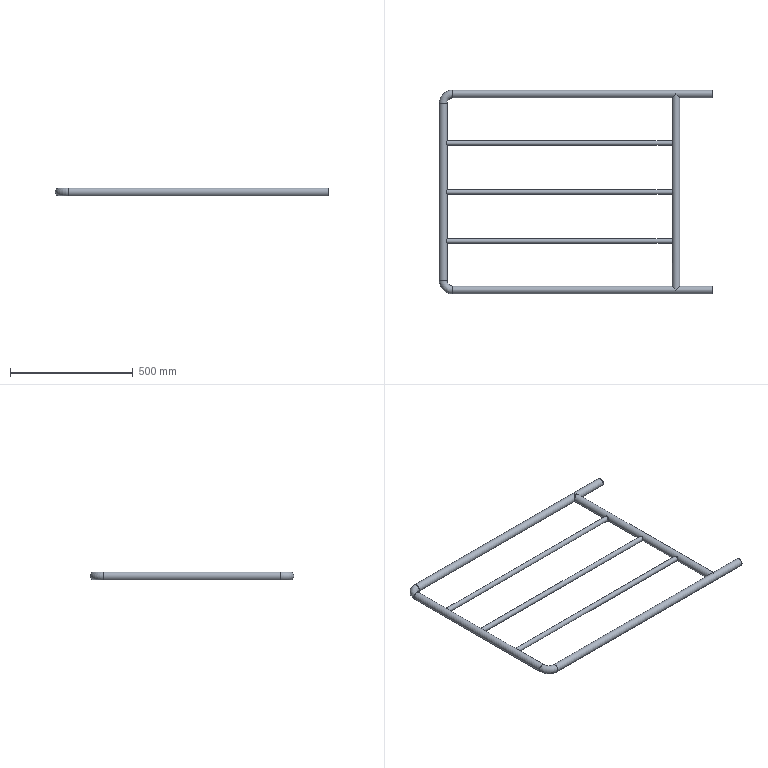Part | STEP file | PN_0003 304 guardrail 800X1100 body-A_Default<As Machined> | 9 solids | 36 faces | box 1116 x 832 x 32 mm | volume 1018076 mm3 | cylinder 22 | plane 10 | torus 4 | commonest cylinder face diameters 32 x12 28 x4 16 x3 20 x3